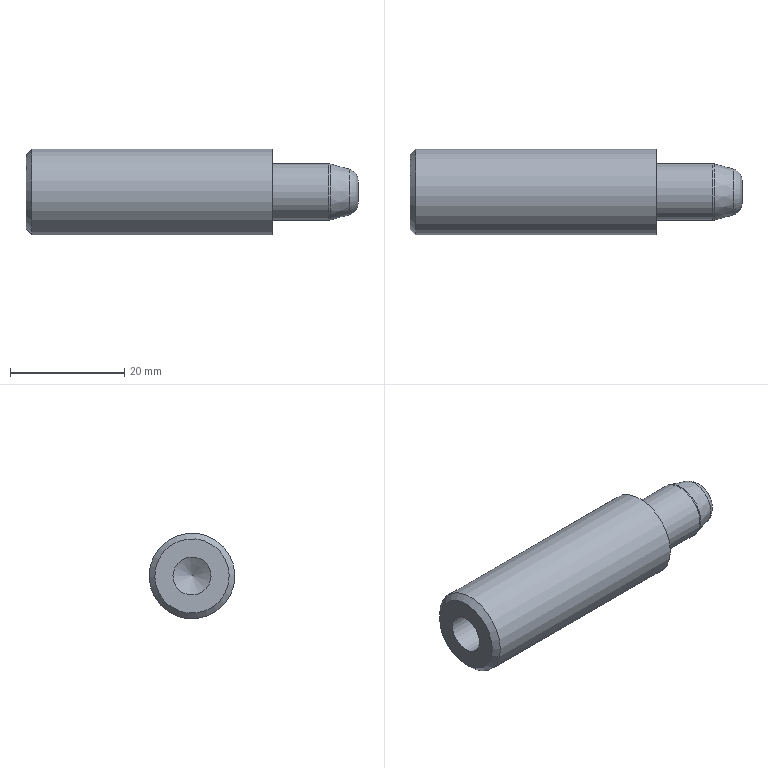Part | STEP file | SN10_013_003_PINO_CONICO | 1 solid | 11 faces | box 58 x 15 x 15 mm | volume 7980 mm3 | cone 3 | plane 3 | cylinder 3 | torus 2 | commonest cylinder face diameters 6.647 x1 9.9 x1 15 x1